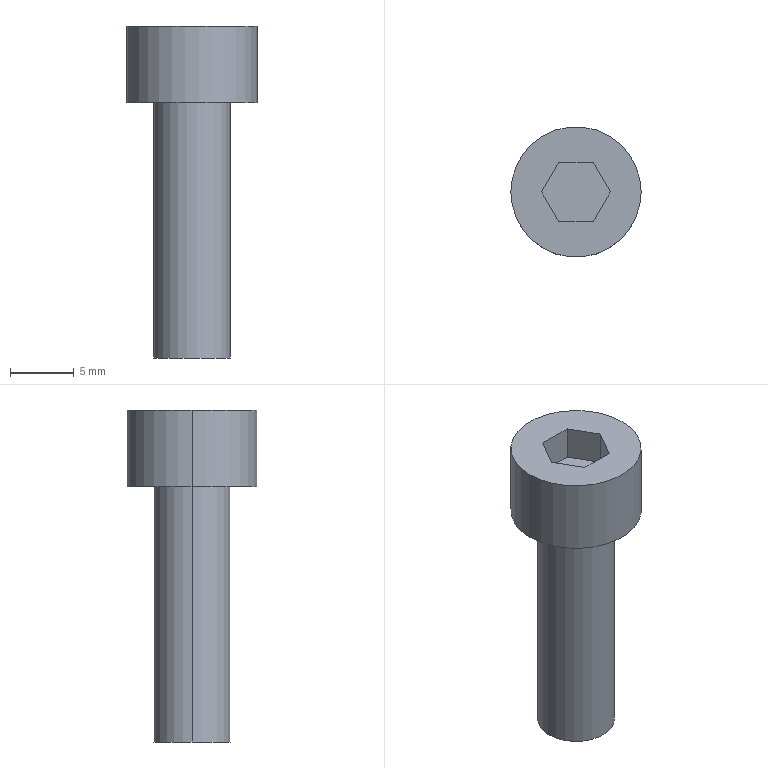Part | SolidWorks | features BaseBody 1 | 1 solid | 14 faces | box 10.2 x 10.2 x 26 mm | volume 1005 mm3 | plane 10 | cylinder 4 | commonest cylinder face diameters 6 x2 10.2 x2
STEP:
#1=CARTESIAN_POINT('',(3.,0.,-20.));
#2=VERTEX_POINT('',#1);
#3=CARTESIAN_POINT('',(-3.,0.,-20.));
#4=VERTEX_POINT('',#3);
#5=CARTESIAN_POINT('',(0.,0.,-20.));
#6=DIRECTION('',(0.,0.,1.));
#7=DIRECTION('',(1.,0.,0.));
#8=AXIS2_PLACEMENT_3D('',#5,#6,#7);
#9=CIRCLE('',#8,3.);
#10=EDGE_CURVE('',#2,#4,#9,.T.);
#11=ORIENTED_EDGE('',*,*,#10,.T.);
#12=CARTESIAN_POINT('',(-3.,0.,0.));
#13=VERTEX_POINT('',#12);
#14=CARTESIAN_POINT('',(-3.,0.,-20.));
#15=DIRECTION('',(0.,0.,1.));
#16=VECTOR('',#15,1000.);
#17=LINE('',#14,#16);
#18=EDGE_CURVE('',#4,#13,#17,.T.);
#19=ORIENTED_EDGE('',*,*,#18,.T.);
#20=CARTESIAN_POINT('',(3.,0.,0.));
#21=VERTEX_POINT('',#20);
#22=CARTESIAN_POINT('',(0.,0.,0.));
#23=DIRECTION('',(0.,0.,-1.));
#24=DIRECTION('',(1.,0.,0.));
#25=AXIS2_PLACEMENT_3D('',#22,#23,#24);
#26=CIRCLE('',#25,3.);
#27=EDGE_CURVE('',#13,#21,#26,.T.);
#28=ORIENTED_EDGE('',*,*,#27,.T.);
#29=CARTESIAN_POINT('',(3.,0.,-20.));
#30=DIRECTION('',(0.,0.,1.));
#31=VECTOR('',#30,1000.);
#32=LINE('',#29,#31);
#33=EDGE_CURVE('',#2,#21,#32,.T.);
#34=ORIENTED_EDGE('',*,*,#33,.F.);
#35=EDGE_LOOP('',(#11,#19,#28,#34));
#36=FACE_OUTER_BOUND('',#35,.T.);
#37=CARTESIAN_POINT('',(0.,0.,-20.));
#38=DIRECTION('',(0.,0.,1.));
#39=DIRECTION('',(1.,0.,0.));
#40=AXIS2_PLACEMENT_3D('',#37,#38,#39);
#41=CYLINDRICAL_SURFACE('',#40,3.);
#42=ADVANCED_FACE('',(#36),#41,.T.);
#43=CARTESIAN_POINT('',(5.1,0.,0.));
#44=VERTEX_POINT('',#43);
#45=CARTESIAN_POINT('',(-5.1,0.,0.));
#46=VERTEX_POINT('',#45);
#47=CARTESIAN_POINT('',(0.,0.,0.));
#48=DIRECTION('',(0.,0.,1.));
#49=DIRECTION('',(1.,0.,0.));
#50=AXIS2_PLACEMENT_3D('',#47,#48,#49);
#51=CIRCLE('',#50,5.1);
#52=EDGE_CURVE('',#44,#46,#51,.T.);
#53=ORIENTED_EDGE('',*,*,#52,.T.);
#54=CARTESIAN_POINT('',(-5.1,0.,6.));
#55=VERTEX_POINT('',#54);
#56=CARTESIAN_POINT('',(-5.1,0.,0.));
#57=DIRECTION('',(0.,0.,1.));
#58=VECTOR('',#57,1000.);
#59=LINE('',#56,#58);
#60=EDGE_CURVE('',#46,#55,#59,.T.);
#61=ORIENTED_EDGE('',*,*,#60,.T.);
#62=CARTESIAN_POINT('',(5.1,0.,6.));
#63=VERTEX_POINT('',#62);
#64=CARTESIAN_POINT('',(0.,0.,6.));
#65=DIRECTION('',(0.,0.,-1.));
#66=DIRECTION('',(1.,0.,0.));
#67=AXIS2_PLACEMENT_3D('',#64,#65,#66);
#68=CIRCLE('',#67,5.1);
#69=EDGE_CURVE('',#55,#63,#68,.T.);
#70=ORIENTED_EDGE('',*,*,#69,.T.);
#71=CARTESIAN_POINT('',(5.1,0.,0.));
#72=DIRECTION('',(0.,0.,1.));
#73=VECTOR('',#72,1000.);
#74=LINE('',#71,#73);
#75=EDGE_CURVE('',#44,#63,#74,.T.);
#76=ORIENTED_EDGE('',*,*,#75,.F.);
#77=EDGE_LOOP('',(#53,#61,#70,#76));
#78=FACE_OUTER_BOUND('',#77,.T.);
#79=CARTESIAN_POINT('',(0.,0.,0.));
#80=DIRECTION('',(0.,0.,1.));
#81=DIRECTION('',(1.,0.,0.));
#82=AXIS2_PLACEMENT_3D('',#79,#80,#81);
#83=CYLINDRICAL_SURFACE('',#82,5.1);
#84=ADVANCED_FACE('',(#78),#83,.T.);
#85=ORIENTED_EDGE('',*,*,#18,.F.);
#86=CARTESIAN_POINT('',(0.,0.,-20.));
#87=DIRECTION('',(0.,0.,1.));
#88=DIRECTION('',(1.,0.,0.));
#89=AXIS2_PLACEMENT_3D('',#86,#87,#88);
#90=CIRCLE('',#89,3.);
#91=EDGE_CURVE('',#4,#2,#90,.T.);
#92=ORIENTED_EDGE('',*,*,#91,.T.);
#93=ORIENTED_EDGE('',*,*,#33,.T.);
#94=CARTESIAN_POINT('',(0.,0.,0.));
#95=DIRECTION('',(0.,0.,-1.));
#96=DIRECTION('',(1.,0.,0.));
#97=AXIS2_PLACEMENT_3D('',#94,#95,#96);
#98=CIRCLE('',#97,3.);
#99=EDGE_CURVE('',#21,#13,#98,.T.);
#100=ORIENTED_EDGE('',*,*,#99,.T.);
#101=EDGE_LOOP('',(#85,#92,#93,#100));
#102=FACE_OUTER_BOUND('',#101,.T.);
#103=CARTESIAN_POINT('',(0.,0.,-20.));
#104=DIRECTION('',(0.,0.,1.));
#105=DIRECTION('',(1.,0.,0.));
#106=AXIS2_PLACEMENT_3D('',#103,#104,#105);
#107=CYLINDRICAL_SURFACE('',#106,3.);
#108=ADVANCED_FACE('',(#102),#107,.T.);
#109=ORIENTED_EDGE('',*,*,#10,.F.);
#110=ORIENTED_EDGE('',*,*,#91,.F.);
#111=EDGE_LOOP('',(#109,#110));
#112=FACE_OUTER_BOUND('',#111,.T.);
#113=CARTESIAN_POINT('',(0.,0.,-20.));
#114=DIRECTION('',(0.,0.,1.));
#115=DIRECTION('',(1.,0.,0.));
#116=AXIS2_PLACEMENT_3D('',#113,#114,#115);
#117=PLANE('',#116);
#118=ADVANCED_FACE('',(#112),#117,.F.);
#119=ORIENTED_EDGE('',*,*,#99,.F.);
#120=ORIENTED_EDGE('',*,*,#27,.F.);
#121=EDGE_LOOP('',(#119,#120));
#122=FACE_BOUND('',#121,.T.);
#123=ORIENTED_EDGE('',*,*,#52,.F.);
#124=CARTESIAN_POINT('',(0.,0.,0.));
#125=DIRECTION('',(0.,0.,1.));
#126=DIRECTION('',(1.,0.,0.));
#127=AXIS2_PLACEMENT_3D('',#124,#125,#126);
#128=CIRCLE('',#127,5.1);
#129=EDGE_CURVE('',#46,#44,#128,.T.);
#130=ORIENTED_EDGE('',*,*,#129,.F.);
#131=EDGE_LOOP('',(#123,#130));
#132=FACE_OUTER_BOUND('',#131,.T.);
#133=CARTESIAN_POINT('',(0.,0.,0.));
#134=DIRECTION('',(0.,0.,1.));
#135=DIRECTION('',(1.,0.,0.));
#136=AXIS2_PLACEMENT_3D('',#133,#134,#135);
#137=PLANE('',#136);
#138=ADVANCED_FACE('',(#122,#132),#137,.F.);
#139=ORIENTED_EDGE('',*,*,#60,.F.);
#140=ORIENTED_EDGE('',*,*,#129,.T.);
#141=ORIENTED_EDGE('',*,*,#75,.T.);
#142=CARTESIAN_POINT('',(0.,0.,6.));
#143=DIRECTION('',(0.,0.,-1.));
#144=DIRECTION('',(1.,0.,0.));
#145=AXIS2_PLACEMENT_3D('',#142,#143,#144);
#146=CIRCLE('',#145,5.1);
#147=EDGE_CURVE('',#63,#55,#146,.T.);
#148=ORIENTED_EDGE('',*,*,#147,.T.);
#149=EDGE_LOOP('',(#139,#140,#141,#148));
#150=FACE_OUTER_BOUND('',#149,.T.);
#151=CARTESIAN_POINT('',(0.,0.,0.));
#152=DIRECTION('',(0.,0.,1.));
#153=DIRECTION('',(1.,0.,0.));
#154=AXIS2_PLACEMENT_3D('',#151,#152,#153);
#155=CYLINDRICAL_SURFACE('',#154,5.1);
#156=ADVANCED_FACE('',(#150),#155,.T.);
#157=CARTESIAN_POINT('',(-1.35,-2.338,6.));
#158=VERTEX_POINT('',#157);
#159=CARTESIAN_POINT('',(-2.7,0.,6.));
#160=VERTEX_POINT('',#159);
#161=CARTESIAN_POINT('',(-1.35,-2.338,6.));
#162=DIRECTION('',(-0.5,0.866,0.));
#163=VECTOR('',#162,1000.);
#164=LINE('',#161,#163);
#165=EDGE_CURVE('',#158,#160,#164,.T.);
#166=ORIENTED_EDGE('',*,*,#165,.T.);
#167=CARTESIAN_POINT('',(-1.35,2.338,6.));
#168=VERTEX_POINT('',#167);
#169=CARTESIAN_POINT('',(-2.7,0.,6.));
#170=DIRECTION('',(0.5,0.866,0.));
#171=VECTOR('',#170,1000.);
#172=LINE('',#169,#171);
#173=EDGE_CURVE('',#160,#168,#172,.T.);
#174=ORIENTED_EDGE('',*,*,#173,.T.);
#175=CARTESIAN_POINT('',(1.35,2.338,6.));
#176=VERTEX_POINT('',#175);
#177=CARTESIAN_POINT('',(0.,2.338,6.));
#178=DIRECTION('',(1.,0.,0.));
#179=VECTOR('',#178,1000.);
#180=LINE('',#177,#179);
#181=EDGE_CURVE('',#168,#176,#180,.T.);
#182=ORIENTED_EDGE('',*,*,#181,.T.);
#183=CARTESIAN_POINT('',(2.7,0.,6.));
#184=VERTEX_POINT('',#183);
#185=CARTESIAN_POINT('',(1.35,2.338,6.));
#186=DIRECTION('',(0.5,-0.866,0.));
#187=VECTOR('',#186,1000.);
#188=LINE('',#185,#187);
#189=EDGE_CURVE('',#176,#184,#188,.T.);
#190=ORIENTED_EDGE('',*,*,#189,.T.);
#191=CARTESIAN_POINT('',(1.35,-2.338,6.));
#192=VERTEX_POINT('',#191);
#193=CARTESIAN_POINT('',(2.7,0.,6.));
#194=DIRECTION('',(-0.5,-0.866,0.));
#195=VECTOR('',#194,1000.);
#196=LINE('',#193,#195);
#197=EDGE_CURVE('',#184,#192,#196,.T.);
#198=ORIENTED_EDGE('',*,*,#197,.T.);
#199=CARTESIAN_POINT('',(0.,-2.338,6.));
#200=DIRECTION('',(-1.,0.,0.));
#201=VECTOR('',#200,1000.);
#202=LINE('',#199,#201);
#203=EDGE_CURVE('',#192,#158,#202,.T.);
#204=ORIENTED_EDGE('',*,*,#203,.T.);
#205=EDGE_LOOP('',(#166,#174,#182,#190,#198,#204));
#206=FACE_BOUND('',#205,.T.);
#207=ORIENTED_EDGE('',*,*,#147,.F.);
#208=ORIENTED_EDGE('',*,*,#69,.F.);
#209=EDGE_LOOP('',(#207,#208));
#210=FACE_OUTER_BOUND('',#209,.T.);
#211=CARTESIAN_POINT('',(0.,0.,6.));
#212=DIRECTION('',(0.,0.,1.));
#213=DIRECTION('',(1.,0.,0.));
#214=AXIS2_PLACEMENT_3D('',#211,#212,#213);
#215=PLANE('',#214);
#216=ADVANCED_FACE('',(#206,#210),#215,.T.);
#217=ORIENTED_EDGE('',*,*,#173,.F.);
#218=CARTESIAN_POINT('',(-2.7,0.,3.3));
#219=VERTEX_POINT('',#218);
#220=CARTESIAN_POINT('',(-2.7,0.,3.3));
#221=DIRECTION('',(0.,0.,-1.));
#222=VECTOR('',#221,1000.);
#223=LINE('',#220,#222);
#224=EDGE_CURVE('',#160,#219,#223,.T.);
#225=ORIENTED_EDGE('',*,*,#224,.T.);
#226=CARTESIAN_POINT('',(-1.35,2.338,3.3));
#227=VERTEX_POINT('',#226);
#228=CARTESIAN_POINT('',(-1.35,2.338,3.3));
#229=DIRECTION('',(0.5,0.866,0.));
#230=VECTOR('',#229,1000.);
#231=LINE('',#228,#230);
#232=EDGE_CURVE('',#219,#227,#231,.T.);
#233=ORIENTED_EDGE('',*,*,#232,.T.);
#234=CARTESIAN_POINT('',(-1.35,2.338,3.3));
#235=DIRECTION('',(0.,0.,1.));
#236=VECTOR('',#235,1000.);
#237=LINE('',#234,#236);
#238=EDGE_CURVE('',#227,#168,#237,.T.);
#239=ORIENTED_EDGE('',*,*,#238,.T.);
#240=EDGE_LOOP('',(#217,#225,#233,#239));
#241=FACE_OUTER_BOUND('',#240,.T.);
#242=CARTESIAN_POINT('',(-1.35,2.338,3.3));
#243=DIRECTION('',(0.866,-0.5,0.));
#244=DIRECTION('',(0.5,0.866,0.));
#245=AXIS2_PLACEMENT_3D('',#242,#243,#244);
#246=PLANE('',#245);
#247=ADVANCED_FACE('',(#241),#246,.T.);
#248=ORIENTED_EDGE('',*,*,#165,.F.);
#249=CARTESIAN_POINT('',(-1.35,-2.338,3.3));
#250=VERTEX_POINT('',#249);
#251=CARTESIAN_POINT('',(-1.35,-2.338,3.3));
#252=DIRECTION('',(0.,0.,-1.));
#253=VECTOR('',#252,1000.);
#254=LINE('',#251,#253);
#255=EDGE_CURVE('',#158,#250,#254,.T.);
#256=ORIENTED_EDGE('',*,*,#255,.T.);
#257=CARTESIAN_POINT('',(-2.7,0.,3.3));
#258=DIRECTION('',(-0.5,0.866,0.));
#259=VECTOR('',#258,1000.);
#260=LINE('',#257,#259);
#261=EDGE_CURVE('',#250,#219,#260,.T.);
#262=ORIENTED_EDGE('',*,*,#261,.T.);
#263=ORIENTED_EDGE('',*,*,#224,.F.);
#264=EDGE_LOOP('',(#248,#256,#262,#263));
#265=FACE_OUTER_BOUND('',#264,.T.);
#266=CARTESIAN_POINT('',(-2.7,0.,3.3));
#267=DIRECTION('',(0.866,0.5,0.));
#268=DIRECTION('',(-0.5,0.866,0.));
#269=AXIS2_PLACEMENT_3D('',#266,#267,#268);
#270=PLANE('',#269);
#271=ADVANCED_FACE('',(#265),#270,.T.);
#272=ORIENTED_EDGE('',*,*,#203,.F.);
#273=CARTESIAN_POINT('',(1.35,-2.338,3.3));
#274=VERTEX_POINT('',#273);
#275=CARTESIAN_POINT('',(1.35,-2.338,3.3));
#276=DIRECTION('',(0.,0.,-1.));
#277=VECTOR('',#276,1000.);
#278=LINE('',#275,#277);
#279=EDGE_CURVE('',#192,#274,#278,.T.);
#280=ORIENTED_EDGE('',*,*,#279,.T.);
#281=CARTESIAN_POINT('',(-1.35,-2.338,3.3));
#282=DIRECTION('',(-1.,0.,0.));
#283=VECTOR('',#282,1000.);
#284=LINE('',#281,#283);
#285=EDGE_CURVE('',#274,#250,#284,.T.);
#286=ORIENTED_EDGE('',*,*,#285,.T.);
#287=ORIENTED_EDGE('',*,*,#255,.F.);
#288=EDGE_LOOP('',(#272,#280,#286,#287));
#289=FACE_OUTER_BOUND('',#288,.T.);
#290=CARTESIAN_POINT('',(-1.35,-2.338,3.3));
#291=DIRECTION('',(0.,1.,0.));
#292=DIRECTION('',(-1.,0.,0.));
#293=AXIS2_PLACEMENT_3D('',#290,#291,#292);
#294=PLANE('',#293);
#295=ADVANCED_FACE('',(#289),#294,.T.);
#296=ORIENTED_EDGE('',*,*,#197,.F.);
#297=CARTESIAN_POINT('',(2.7,0.,3.3));
#298=VERTEX_POINT('',#297);
#299=CARTESIAN_POINT('',(2.7,0.,3.3));
#300=DIRECTION('',(0.,0.,-1.));
#301=VECTOR('',#300,1000.);
#302=LINE('',#299,#301);
#303=EDGE_CURVE('',#184,#298,#302,.T.);
#304=ORIENTED_EDGE('',*,*,#303,.T.);
#305=CARTESIAN_POINT('',(1.35,-2.338,3.3));
#306=DIRECTION('',(-0.5,-0.866,0.));
#307=VECTOR('',#306,1000.);
#308=LINE('',#305,#307);
#309=EDGE_CURVE('',#298,#274,#308,.T.);
#310=ORIENTED_EDGE('',*,*,#309,.T.);
#311=ORIENTED_EDGE('',*,*,#279,.F.);
#312=EDGE_LOOP('',(#296,#304,#310,#311));
#313=FACE_OUTER_BOUND('',#312,.T.);
#314=CARTESIAN_POINT('',(1.35,-2.338,3.3));
#315=DIRECTION('',(-0.866,0.5,0.));
#316=DIRECTION('',(-0.5,-0.866,0.));
#317=AXIS2_PLACEMENT_3D('',#314,#315,#316);
#318=PLANE('',#317);
#319=ADVANCED_FACE('',(#313),#318,.T.);
#320=ORIENTED_EDGE('',*,*,#189,.F.);
#321=CARTESIAN_POINT('',(1.35,2.338,3.3));
#322=VERTEX_POINT('',#321);
#323=CARTESIAN_POINT('',(1.35,2.338,3.3));
#324=DIRECTION('',(0.,0.,-1.));
#325=VECTOR('',#324,1000.);
#326=LINE('',#323,#325);
#327=EDGE_CURVE('',#176,#322,#326,.T.);
#328=ORIENTED_EDGE('',*,*,#327,.T.);
#329=CARTESIAN_POINT('',(2.7,0.,3.3));
#330=DIRECTION('',(0.5,-0.866,0.));
#331=VECTOR('',#330,1000.);
#332=LINE('',#329,#331);
#333=EDGE_CURVE('',#322,#298,#332,.T.);
#334=ORIENTED_EDGE('',*,*,#333,.T.);
#335=ORIENTED_EDGE('',*,*,#303,.F.);
#336=EDGE_LOOP('',(#320,#328,#334,#335));
#337=FACE_OUTER_BOUND('',#336,.T.);
#338=CARTESIAN_POINT('',(2.7,0.,3.3));
#339=DIRECTION('',(-0.866,-0.5,0.));
#340=DIRECTION('',(0.5,-0.866,0.));
#341=AXIS2_PLACEMENT_3D('',#338,#339,#340);
#342=PLANE('',#341);
#343=ADVANCED_FACE('',(#337),#342,.T.);
#344=ORIENTED_EDGE('',*,*,#181,.F.);
#345=ORIENTED_EDGE('',*,*,#238,.F.);
#346=CARTESIAN_POINT('',(1.35,2.338,3.3));
#347=DIRECTION('',(1.,0.,0.));
#348=VECTOR('',#347,1000.);
#349=LINE('',#346,#348);
#350=EDGE_CURVE('',#227,#322,#349,.T.);
#351=ORIENTED_EDGE('',*,*,#350,.T.);
#352=ORIENTED_EDGE('',*,*,#327,.F.);
#353=EDGE_LOOP('',(#344,#345,#351,#352));
#354=FACE_OUTER_BOUND('',#353,.T.);
#355=CARTESIAN_POINT('',(1.35,2.338,3.3));
#356=DIRECTION('',(0.,-1.,0.));
#357=DIRECTION('',(0.,0.,-1.));
#358=AXIS2_PLACEMENT_3D('',#355,#356,#357);
#359=PLANE('',#358);
#360=ADVANCED_FACE('',(#354),#359,.T.);
#361=ORIENTED_EDGE('',*,*,#285,.F.);
#362=ORIENTED_EDGE('',*,*,#309,.F.);
#363=ORIENTED_EDGE('',*,*,#333,.F.);
#364=ORIENTED_EDGE('',*,*,#350,.F.);
#365=ORIENTED_EDGE('',*,*,#232,.F.);
#366=ORIENTED_EDGE('',*,*,#261,.F.);
#367=EDGE_LOOP('',(#361,#362,#363,#364,#365,#366));
#368=FACE_OUTER_BOUND('',#367,.T.);
#369=CARTESIAN_POINT('',(0.,0.,3.3));
#370=DIRECTION('',(0.,0.,1.));
#371=DIRECTION('',(1.,0.,0.));
#372=AXIS2_PLACEMENT_3D('',#369,#370,#371);
#373=PLANE('',#372);
#374=ADVANCED_FACE('',(#368),#373,.T.);
#375=CLOSED_SHELL('',(#42,#84,#108,#118,#138,#156,#216,#247,#271,#295,#319,#343,#360,#374));
#376=MANIFOLD_SOLID_BREP('',#375);
#377=CARTESIAN_POINT('',(0.,0.,0.));
#378=DIRECTION('',(0.,0.,1.));
#379=DIRECTION('',(1.,0.,0.));
#380=AXIS2_PLACEMENT_3D('',#377,#378,#379);
#381=(LENGTH_UNIT()NAMED_UNIT(*)SI_UNIT(.MILLI.,.METRE.));
#382=UNCERTAINTY_MEASURE_WITH_UNIT(LENGTH_MEASURE(0.00001),#381,'','');
#383=(NAMED_UNIT(*)PLANE_ANGLE_UNIT()SI_UNIT($,.RADIAN.));
#384=(NAMED_UNIT(*)SI_UNIT($,.STERADIAN.)SOLID_ANGLE_UNIT());
#385=(GEOMETRIC_REPRESENTATION_CONTEXT(3)GLOBAL_UNCERTAINTY_ASSIGNED_CONTEXT((#382))GLOBAL_UNIT_ASSIGNED_CONTEXT((#381,#383,#384))REPRESENTATION_CONTEXT('',''));
#386=ADVANCED_BREP_SHAPE_REPRESENTATION('',(#376,#380),#385);